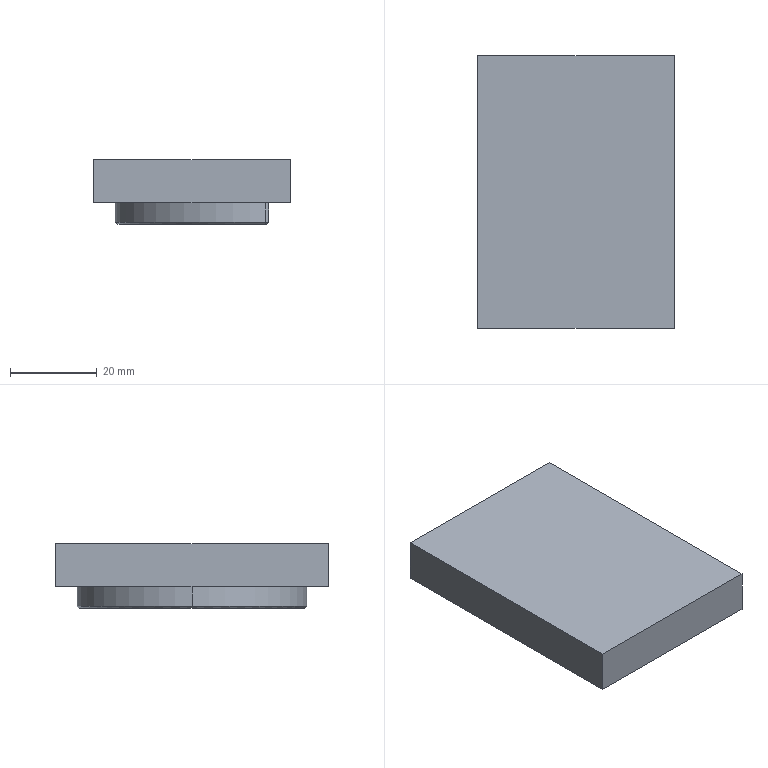NC program | NX | posted with a generic post | part box 45.394 x 63 x 15 mm
Whole program:
N10 G17 G21 G94 G90
(FLOOR_WALL , TOOL : D80)
N12 T19 M6
N14 G54
N16 G17 G0 G90 X-71.5 Y0. S5000 M3
N18 G43 Z30. H19
N20 Z3.
N22 G94 G1 Z0. F1200.
N24 X-68.5
N26 X68.5
N28 X71.5
N30 Z3.
N32 G0 Z30.
N34 M5
(CAVITY_MILL , TOOL : D10)
N36 T15 M6
N38 G54
N40 G17 G0 G90 X5.485 Y-28.695 S9500 M3
N42 G43 Z30. H15
N44 Z1.35
N46 G94 G1 Z-1.65 F1000.
N48 X0.866 Y-20.695
N50 G3 X0. Y-20.195 R1.
N52 G1 X-17.653 F3500.
N54 X-18.655 Y-21.39
N56 G2 X-31.189 Y-18.957 R7.3
N58 X-28.996 Y6.529 R32.8
N60 G1 Y19.7
N62 G2 X-28.501 Y20.195 R0.495
N64 G1 X-15.329
N66 G2 X15.329 Y20.195 R32.8
N68 G1 X28.501
N70 G2 X28.996 Y19.7 R0.495
N72 G1 Y6.529
N74 G2 X31.189 Y-18.957 R32.8
N76 X18.655 Y-21.39 R7.3
N78 G1 X17.653 Y-20.195
N80 X0.
N82 Y-14.195
N84 X-13.178
N86 G3 X-12.194 Y-9.201 R11.3
N88 G2 X12.194 Y-9.201 R-12.2
N90 G3 X13.178 Y-14.195 R11.3
N92 G1 X14.273 Y-13.704
N94 G2 X13.393 Y-9.24 R10.1
N96 G3 X-13.393 Y-9.24 R-13.4
N98 G2 X-15.75 Y-16.061 R10.1
N100 G1 X-19.574 Y-20.618
N102 G2 X-30.048 Y-18.586 R6.1
N104 X30.048 Y-18.586 R-31.6
N106 X19.574 Y-20.618 R6.1
N108 G1 X15.75 Y-16.061
N110 G2 X14.273 Y-13.704 R10.1
N112 G1 X13.178 Y-14.195
N114 X0.
N116 Y-8.195
N118 X-6.17
N120 G2 X6.17 Y-8.195 R6.2
N122 G1 X0.
N124 G3 X-0.866 Y-8.695 R1.
N126 G1 Z1.35
N128 G0 X5.485 Y-28.695 Z-0.3
N130 G1 Z-3.3 F1000.
N132 X0.866 Y-20.695
N134 G3 X0. Y-20.195 R1.
N136 G1 X-17.653 F3500.
N138 X-18.655 Y-21.39
N140 G2 X-31.189 Y-18.957 R7.3
N142 X-28.997 Y6.527 R32.8
N144 G1 Y19.699
N146 G2 X-28.501 Y20.195 R0.496
N148 G1 X-15.328
N150 G2 X15.328 Y20.195 R32.8
N152 G1 X28.501
N154 G2 X28.997 Y19.699 R0.496
N156 G1 Y6.527
N158 G2 X31.189 Y-18.957 R32.8
N160 X18.655 Y-21.39 R7.3
N162 G1 X17.653 Y-20.195
N164 X0.
N166 Y-14.195
N168 X-13.178
N170 G3 X-12.194 Y-9.201 R11.3
N172 G2 X12.194 Y-9.201 R-12.2
N174 G3 X13.178 Y-14.195 R11.3
N176 G1 X14.273 Y-13.704
N178 G2 X13.393 Y-9.24 R10.1
N180 G3 X-13.393 Y-9.24 R-13.4
N182 G2 X-15.75 Y-16.061 R10.1
N184 G1 X-19.574 Y-20.618
N186 G2 X-30.048 Y-18.586 R6.1
N188 X30.048 Y-18.586 R-31.6
N190 X19.574 Y-20.618 R6.1
N192 G1 X15.75 Y-16.061
N194 G2 X14.273 Y-13.704 R10.1
N196 G1 X13.178 Y-14.195
N198 X0.
N200 Y-8.195
N202 X-6.17
N204 G2 X6.17 Y-8.195 R6.2
N206 G1 X0.
N208 G3 X-0.866 Y-8.695 R1.
N210 G1 Z-0.3
N212 G0 X5.485 Y-28.696 Z-1.975
N214 G1 Z-4.975 F1000.
N216 X0.866 Y-20.696
N218 G3 X0. Y-20.196 R1.
N220 G1 X-17.653 F3500.
N222 X-18.655 Y-21.39
N224 G2 X-31.189 Y-18.957 R7.3
N226 X-28.998 Y6.526 R32.8
N228 G1 Y19.699
N230 G2 X-28.501 Y20.196 R0.497
N232 G1 X-15.327
N234 G2 X15.327 Y20.196 R32.8
N236 G1 X28.501
N238 G2 X28.998 Y19.699 R0.497
N240 G1 Y6.526
N242 G2 X31.189 Y-18.957 R32.8
N244 X18.655 Y-21.39 R7.3
N246 G1 X17.653 Y-20.196
N248 X0.
N250 Y-14.196
N252 X-13.178
N254 G3 X-12.194 Y-9.201 R11.3
N256 G2 X12.194 Y-9.201 R-12.2
N258 G3 X13.178 Y-14.196 R11.3
N260 G1 X14.273 Y-13.704
N262 G2 X13.393 Y-9.24 R10.1
N264 G3 X-13.393 Y-9.24 R-13.4
N266 G2 X-15.75 Y-16.061 R10.1
N268 G1 X-19.574 Y-20.618
N270 G2 X-30.048 Y-18.586 R6.1
N272 X30.048 Y-18.586 R-31.6
N274 X19.574 Y-20.618 R6.1
N276 G1 X15.75 Y-16.061
N278 G2 X14.273 Y-13.704 R10.1
N280 G1 X13.178 Y-14.196
N282 X0.
N284 Y-8.196
N286 X-6.17
N288 G2 X6.17 Y-8.196 R6.2
N290 G1 X0.
N292 G3 X-0.866 Y-8.696 R1.
N294 G1 Z-1.975
N296 G0 X5.485 Y-28.696 Z-3.65
N298 G1 Z-6.65 F1000.
N300 X0.866 Y-20.696
N302 G3 X0. Y-20.196 R1.
N304 G1 X-17.654 F3500.
N306 X-18.655 Y-21.39
N308 G2 X-31.189 Y-18.957 R7.3
N310 X-28.998 Y6.525 R32.8
N312 G1 Y19.699
N314 G2 X-28.501 Y20.196 R0.497
N316 G1 X-15.326
N318 G2 X15.326 Y20.196 R32.8
N320 G1 X28.501
N322 G2 X28.998 Y19.699 R0.497
N324 G1 Y6.525
N326 G2 X31.189 Y-18.957 R32.8
N328 X18.655 Y-21.39 R7.3
N330 G1 X17.654 Y-20.196
N332 X0.
N334 Y-14.196
N336 X-13.178
N338 G3 X-12.194 Y-9.201 R11.3
N340 G2 X12.194 Y-9.201 R-12.2
N342 G3 X13.178 Y-14.196 R11.3
N344 G1 X14.273 Y-13.705
N346 G2 X13.393 Y-9.24 R10.1
N348 G3 X-13.393 Y-9.24 R-13.4
N350 G2 X-15.75 Y-16.061 R10.1
N352 G1 X-19.574 Y-20.618
N354 G2 X-30.048 Y-18.586 R6.1
N356 X30.048 Y-18.586 R-31.6
N358 X19.574 Y-20.618 R6.1
N360 G1 X15.75 Y-16.061
N362 G2 X14.273 Y-13.705 R10.1
N364 G1 X13.178 Y-14.196
N366 X0.
N368 Y-8.196
N370 X-6.17
N372 G2 X6.17 Y-8.196 R6.2
N374 G1 X0.
N376 G3 X-0.866 Y-8.696 R1.
N378 G1 Z-3.65
N380 G0 X5.485 Y-28.697 Z-5.325
N382 G1 Z-8.325 F1000.
N384 X0.866 Y-20.697
N386 G3 X0. Y-20.197 R1.
N388 G1 X-17.654 F3500.
N390 X-18.655 Y-21.39
N392 G2 X-31.189 Y-18.957 R7.3
N394 X-28.999 Y6.524 R32.8
N396 G1 Y19.699
N398 G2 X-28.501 Y20.197 R0.498
N400 G1 X-15.325
N402 G2 X15.325 Y20.197 R32.8
N404 G1 X28.501
N406 G2 X28.999 Y19.699 R0.498
N408 G1 Y6.524
N410 G2 X31.189 Y-18.957 R32.8
N412 X18.655 Y-21.39 R7.3
N414 G1 X17.654 Y-20.197
N416 X0.
N418 Y-14.197
N420 X-13.179
N422 G3 X-12.194 Y-9.201 R11.3
N424 G2 X12.194 Y-9.201 R-12.2
N426 G3 X13.179 Y-14.197 R11.3
N428 G1 X14.273 Y-13.705
N430 G2 X13.393 Y-9.24 R10.1
N432 G3 X-13.393 Y-9.24 R-13.4
N434 G2 X-15.75 Y-16.061 R10.1
N436 G1 X-19.574 Y-20.618
N438 G2 X-30.048 Y-18.586 R6.1
N440 X30.048 Y-18.586 R-31.6
N442 X19.574 Y-20.618 R6.1
N444 G1 X15.75 Y-16.061
N446 G2 X14.273 Y-13.705 R10.1
N448 G1 X13.179 Y-14.197
N450 X0.
N452 Y-8.197
N454 X-6.17
N456 G2 X6.17 Y-8.197 R6.2
N458 G1 X0.
N460 G3 X-0.866 Y-8.697 R1.
N462 G1 Z-5.325
N464 G0 X5.485 Y-28.697 Z-7.
N466 G1 Z-10. F1000.
N468 X0.866 Y-20.697
N470 G3 X0. Y-20.197 R1.
N472 G1 X-17.655 F3500.
N474 X-18.655 Y-21.39
N476 G2 X-31.189 Y-18.957 R7.3
N478 X-29. Y6.522 R32.8
N480 G1 Y19.698
N482 G2 X-28.501 Y20.197 R0.499
N484 G1 X-15.324
N486 G2 X15.324 Y20.197 R32.8
N488 G1 X28.501
N490 G2 X29. Y19.698 R0.499
N492 G1 Y6.522
N494 G2 X31.189 Y-18.957 R32.8
N496 X18.655 Y-21.39 R7.3
N498 G1 X17.655 Y-20.197
N500 X0.
N502 Y-14.197
N504 X-13.179
N506 G3 X-12.194 Y-9.201 R11.3
N508 G2 X12.194 Y-9.201 R-12.2
N510 G3 X13.179 Y-14.197 R11.3
N512 G1 X14.274 Y-13.706
N514 G2 X13.393 Y-9.24 R10.1
N516 G3 X-13.393 Y-9.24 R-13.4
N518 G2 X-15.75 Y-16.061 R10.1
N520 G1 X-19.574 Y-20.618
N522 G2 X-30.048 Y-18.586 R6.1
N524 X30.048 Y-18.586 R-31.6
N526 X19.574 Y-20.618 R6.1
N528 G1 X15.75 Y-16.061
N530 G2 X14.274 Y-13.706 R10.1
N532 G1 X13.179 Y-14.197
N534 X0.
N536 Y-8.197
N538 X-6.17
N540 G2 X6.17 Y-8.197 R6.2
N542 G1 X0.
N544 G3 X-0.866 Y-8.697 R1.
N546 G1 Z-7.
N548 G0 Z30.
N550 M5
(ZLEVEL_PROFILE_COPY , TOOL : D10JING)
N552 T14 M6
N554 G54
N556 G17 G0 G90 X-0.362 Y4.698 S9500 M3
N558 G43 Z30. H14
N560 Z-8.5
N562 G94 G1 X-0.876 Y4.699 Z-8.527 F1000.
N564 X-3.332 Y4.311 Z-8.657
N566 X-5.675 Y3.48 Z-8.788
N568 X-7.826 Y2.234 Z-8.918
N570 X-9.713 Y0.616 Z-9.048
N572 X-11.273 Y-1.32 Z-9.178
N574 X-12.451 Y-3.509 Z-9.309
N576 X-13.21 Y-5.877 Z-9.439
N578 X-13.522 Y-8.343 Z-9.569
N580 X-13.493 Y-9.243 Z-9.616
N582 X-13.468 Y-10.018 Z-9.657
N584 X-13.737 Y-11.922 Z-9.758
N586 X-14.365 Y-13.739 Z-9.859
N588 X-15.329 Y-15.403 Z-9.959
N590 X-15.827 Y-15.997 Z-10.
N592 X-19.651 Y-20.554 F1500.
N594 G2 X-29.952 Y-18.555 R6.
N596 X29.952 Y-18.555 R-31.5
N598 X19.651 Y-20.554 R6.
N600 G1 X15.827 Y-15.997
N602 G2 X13.493 Y-9.243 R10.
N604 G3 X-13.493 Y-9.243 R-13.5
N606 G2 X-15.827 Y-15.997 R10.
N608 G1 Z-8.5
N610 G0 Z30.
N612 M5
(SPOT_DRILLING , TOOL : D6A45)
N614 T01 M6
N616 G54
N618 G17 G0 G90 X22. Y-8.803 S9500 M3
N620 G43 Z30. H1
N622 G94 G82 G98 Z-1. F250. P200 R3.
N624 X15.556 Y6.754
N626 X-15.556
N628 X-22. Y-8.803
N630 G80
N632 G0 X-22. Y-8.803 Z30.
N634 M5
(DRILLING_COPY_COPY , TOOL : 3.5ZT)
N636 T07 M6
N638 G54
N640 G17 G0 G90 X22. Y-8.803 S2500 M3
N642 G43 Z30. H7
N644 G94 G83 G98 Z-12.521 F200. Q2. R3.
N646 X15.556 Y6.754
N648 X-15.556
N650 X-22. Y-8.803
N652 G80
N654 G0 X-22. Y-8.803 Z30.
N656 M5
(HOLE_MILLING_2 , TOOL : D4)
N658 T11 M6
N660 G54
N662 G17 G0 G90 X-15.556 Y6.754 S9500 M3
N664 G43 Z30. H11
N666 Z0.5
N668 G94 G3 X-16.056 Y6.254 R0.5 F1250.
N670 X-15.556 Y5.754 R0.5
N672 X-15.556 Y5.754 Z0.1 I0. J1.
N674 X-15.556 Y5.754 Z-0.3 I0. J1.
N676 X-15.556 Y5.754 Z-0.7 I0. J1.
N678 X-15.556 Y5.754 Z-1.1 I0. J1.
N680 X-15.556 Y5.754 Z-1.5 I0. J1.
N682 X-15.556 Y5.754 Z-1.9 I0. J1.
N684 X-15.556 Y5.754 Z-2.3 I0. J1.
N686 X-15.556 Y5.754 Z-2.7 I0. J1.
N688 X-15.556 Y5.754 Z-3.1 I0. J1.
N690 X-16.556 Y6.754 Z-3.4 R-1.
N692 X-15.556 Y5.754 R1.
N694 X-16.556 Y6.754 R-1.
N696 X-16.056 Y6.254 R0.5
N698 X-15.556 Y6.754 R0.5
N700 G0 Z30.
N702 X-22. Y-8.803
N704 Z0.5
N706 G3 X-22.5 Y-9.303 R0.5
N708 X-22. Y-9.803 R0.5
N710 X-22. Y-9.803 Z0.1 I0. J1.
N712 X-22. Y-9.803 Z-0.3 I0. J1.
N714 X-22. Y-9.803 Z-0.7 I0. J1.
N716 X-22. Y-9.803 Z-1.1 I0. J1.
N718 X-22. Y-9.803 Z-1.5 I0. J1.
N720 X-22. Y-9.803 Z-1.9 I0. J1.
N722 X-22. Y-9.803 Z-2.3 I0. J1.
N724 X-22. Y-9.803 Z-2.7 I0. J1.
N726 X-22. Y-9.803 Z-3.1 I0. J1.
N728 X-23. Y-8.803 Z-3.4 R-1.
N730 X-22. Y-9.803 R1.
N732 X-23. Y-8.803 R-1.
N734 X-22.5 Y-9.303 R0.5
N736 X-22. Y-8.803 R0.5
N738 G0 Z30.
N740 X15.556 Y6.754
N742 Z0.5
N744 G3 X15.056 Y6.254 R0.5
N746 X15.556 Y5.754 R0.5
N748 X15.556 Y5.754 Z0.1 I0. J1.
N750 X15.556 Y5.754 Z-0.3 I0. J1.
N752 X15.556 Y5.754 Z-0.7 I0. J1.
N754 X15.556 Y5.754 Z-1.1 I0. J1.
N756 X15.556 Y5.754 Z-1.5 I0. J1.
N758 X15.556 Y5.754 Z-1.9 I0. J1.
N760 X15.556 Y5.754 Z-2.3 I0. J1.
N762 X15.556 Y5.754 Z-2.7 I0. J1.
N764 X15.556 Y5.754 Z-3.1 I0. J1.
N766 X14.556 Y6.754 Z-3.4 R-1.
N768 X15.556 Y5.754 R1.
N770 X14.556 Y6.754 R-1.
N772 X15.056 Y6.254 R0.5
N774 X15.556 Y6.754 R0.5
N776 G0 Z30.
N778 X22. Y-8.803
N780 Z0.5
N782 G3 X21.5 Y-9.303 R0.5
N784 X22. Y-9.803 R0.5
N786 X22. Y-9.803 Z0.1 I0. J1.
N788 X22. Y-9.803 Z-0.3 I0. J1.
N790 X22. Y-9.803 Z-0.7 I0. J1.
N792 X22. Y-9.803 Z-1.1 I0. J1.
N794 X22. Y-9.803 Z-1.5 I0. J1.
N796 X22. Y-9.803 Z-1.9 I0. J1.
N798 X22. Y-9.803 Z-2.3 I0. J1.
N800 X22. Y-9.803 Z-2.7 I0. J1.
N802 X22. Y-9.803 Z-3.1 I0. J1.
N804 X21. Y-8.803 Z-3.4 R-1.
N806 X22. Y-9.803 R1.
N808 X21. Y-8.803 R-1.
N810 X21.5 Y-9.303 R0.5
N812 X22. Y-8.803 R0.5
N814 G0 Z30.
N816 M5
(PLANAR_PROFILE , TOOL : D6A45)
N818 T01 M6
N820 G54
N822 G17 G0 G90 X20.915 Y-8.839 S9500 M3
N824 G43 Z30. H1
N826 Z0.5
N828 G94 G1 Z-1. F1500.
N830 X20.31 Y-8.663
N832 G3 X19.727 Y-8.805 R0.6
N834 G2 X20.009 Y-9.291 R1.
N836 G3 X20.008 Y-8.318 R-2.05
N838 G2 X19.727 Y-8.805 R1.
N840 G3 X20.311 Y-8.946 R0.6
N842 G1 X20.915 Y-8.768
N844 Z0.5
N846 G0 Z30.
N848 X14.809 Y5.964
N850 Z0.5
N852 G1 Z-1.
N854 X14.261 Y5.662
N856 G3 X13.951 Y5.148 R0.6
N858 G2 X14.49 Y5.003 R1.
N860 G3 X13.805 Y5.688 R-2.05
N862 G2 X13.951 Y5.148 R1.
N864 G3 X14.465 Y5.458 R0.6
N866 G1 X14.767 Y6.006
N868 Z0.5
N870 G0 Z30.
N872 X23.023 Y-18.819
N874 Z0.5
N876 G1 Z-1.
N878 X23.241 Y-18.22
N880 G3 X23.136 Y-17.629 R0.6
N882 G1 X19.313 Y-13.072
N884 G2 X18.038 Y-9.52 R5.45
N886 X18.347 Y-8.806 R1.
N888 X18.037 Y-8.12 R1.
N890 G3 X13.237 Y3.469 R18.05
N892 G2 X12.971 Y4.168 R1.
N894 X12.271 Y4.434 R1.
N896 G3 X-12.271 Y4.434 R18.05
N898 G2 X-12.971 Y4.168 R1.
N900 X-13.237 Y3.469 R1.
N902 G3 X-18.037 Y-8.12 R18.05
N904 G2 X-18.347 Y-8.806 R1.
N906 X-18.038 Y-9.52 R1.
N908 X-19.313 Y-13.072 R5.45
N910 G1 X-23.136 Y-17.629
N912 G2 X-25.626 Y-17.146 R1.45
N914 X25.626 Y-17.146 R-26.95
N916 X23.136 Y-17.629 R1.45
N918 G3 X22.573 Y-17.424 R0.6
N920 G1 X21.777 Y-17.564
N922 Z0.5
N924 G0 Z30.
N926 X-14.767 Y6.006
N928 Z0.5
N930 G1 Z-1.
N932 X-14.465 Y5.458
N934 G3 X-13.951 Y5.148 R0.6
N936 G2 X-13.805 Y5.688 R1.
N938 G3 X-14.49 Y5.003 R-2.05
N940 G2 X-13.951 Y5.148 R1.
N942 G3 X-14.261 Y5.662 R0.6
N944 G1 X-14.809 Y5.964
N946 Z0.5
N948 G0 Z30.
N950 X-20.915 Y-8.768
N952 Z0.5
N954 G1 Z-1.
N956 X-20.311 Y-8.946
N958 G3 X-19.727 Y-8.805 R0.6
N960 G2 X-20.008 Y-8.318 R1.
N962 G3 X-20.009 Y-9.291 R-2.05
N964 G2 X-19.727 Y-8.805 R1.
N966 G3 X-20.31 Y-8.663 R0.6
N968 G1 X-20.915 Y-8.839
N970 Z0.5
N972 G0 Z30.
N974 M5
N976 M2